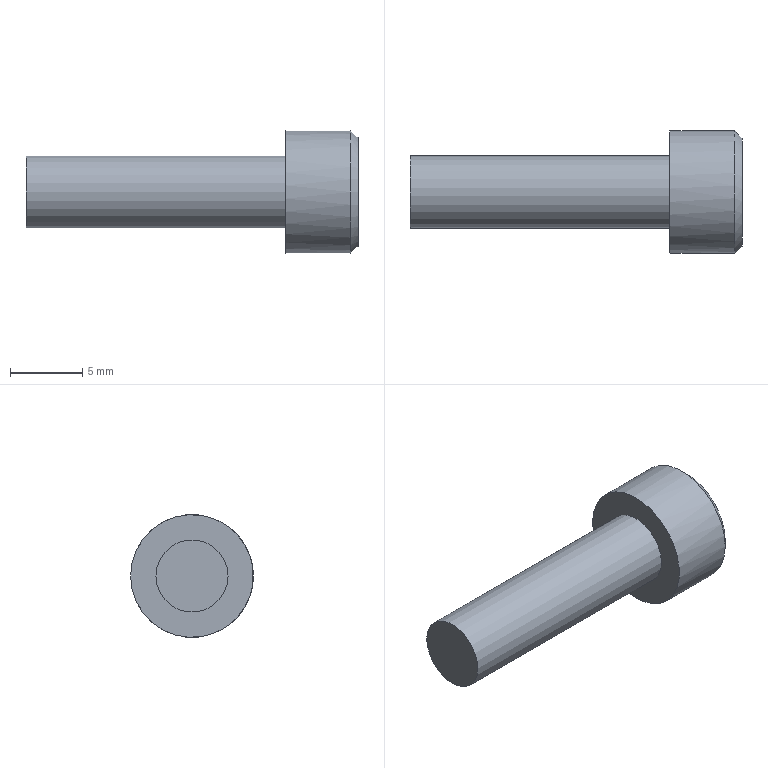Part | NX | features 5003_312_CB5-18 2 | 1 solid | 19 faces | box 23 x 8.5 x 8.5 mm | volume 594.272 mm3 | plane 15 | cylinder 2 | cone 2 | commonest cylinder face diameters 5 x1 8.5 x1
STEP:
#1=CARTESIAN_POINT('',(227.825,81.75,-47.));
#2=VERTEX_POINT('',#1);
#3=CARTESIAN_POINT('',(227.825,85.5,-47.));
#4=DIRECTION('',(-1.,0.,0.));
#5=DIRECTION('',(0.,-1.,0.));
#6=AXIS2_PLACEMENT_3D('',#3,#4,#5);
#7=CIRCLE('',#6,3.75);
#8=EDGE_CURVE('',#2,#2,#7,.F.);
#9=ORIENTED_EDGE('',*,*,#8,.T.);
#10=EDGE_LOOP('',(#9));
#11=FACE_BOUND('',#10,.T.);
#12=CARTESIAN_POINT('',(227.825,85.5,-49.309));
#13=VERTEX_POINT('',#12);
#14=CARTESIAN_POINT('',(227.825,87.5,-48.155));
#15=VERTEX_POINT('',#14);
#16=CARTESIAN_POINT('',(227.825,85.5,-49.309));
#17=DIRECTION('',(0.,0.866,0.5));
#18=VECTOR('',#17,1000.);
#19=LINE('',#16,#18);
#20=EDGE_CURVE('',#13,#15,#19,.T.);
#21=ORIENTED_EDGE('',*,*,#20,.F.);
#22=CARTESIAN_POINT('',(227.825,83.5,-48.155));
#23=VERTEX_POINT('',#22);
#24=CARTESIAN_POINT('',(227.825,83.5,-48.155));
#25=DIRECTION('',(0.,0.866,-0.5));
#26=VECTOR('',#25,1000.);
#27=LINE('',#24,#26);
#28=EDGE_CURVE('',#23,#13,#27,.T.);
#29=ORIENTED_EDGE('',*,*,#28,.F.);
#30=CARTESIAN_POINT('',(227.825,83.5,-45.845));
#31=VERTEX_POINT('',#30);
#32=CARTESIAN_POINT('',(227.825,83.5,-45.845));
#33=DIRECTION('',(0.,0.,-1.));
#34=VECTOR('',#33,1000.);
#35=LINE('',#32,#34);
#36=EDGE_CURVE('',#31,#23,#35,.T.);
#37=ORIENTED_EDGE('',*,*,#36,.F.);
#38=CARTESIAN_POINT('',(227.825,85.5,-44.691));
#39=VERTEX_POINT('',#38);
#40=CARTESIAN_POINT('',(227.825,85.5,-44.691));
#41=DIRECTION('',(0.,-0.866,-0.5));
#42=VECTOR('',#41,1000.);
#43=LINE('',#40,#42);
#44=EDGE_CURVE('',#39,#31,#43,.T.);
#45=ORIENTED_EDGE('',*,*,#44,.F.);
#46=CARTESIAN_POINT('',(227.825,87.5,-45.845));
#47=VERTEX_POINT('',#46);
#48=CARTESIAN_POINT('',(227.825,87.5,-45.845));
#49=DIRECTION('',(0.,-0.866,0.5));
#50=VECTOR('',#49,1000.);
#51=LINE('',#48,#50);
#52=EDGE_CURVE('',#47,#39,#51,.T.);
#53=ORIENTED_EDGE('',*,*,#52,.F.);
#54=CARTESIAN_POINT('',(227.825,87.5,-48.155));
#55=DIRECTION('',(0.,0.,1.));
#56=VECTOR('',#55,1000.);
#57=LINE('',#54,#56);
#58=EDGE_CURVE('',#15,#47,#57,.T.);
#59=ORIENTED_EDGE('',*,*,#58,.F.);
#60=EDGE_LOOP('',(#21,#29,#37,#45,#53,#59));
#61=FACE_BOUND('',#60,.T.);
#62=CARTESIAN_POINT('',(227.825,85.5,-42.75));
#63=DIRECTION('',(-1.,0.,0.));
#64=DIRECTION('',(0.,-1.,0.));
#65=AXIS2_PLACEMENT_3D('',#62,#63,#64);
#66=PLANE('',#65);
#67=ADVANCED_FACE('',(#11,#61),#66,.F.);
#68=CARTESIAN_POINT('',(204.825,88.,-47.));
#69=VERTEX_POINT('',#68);
#70=CARTESIAN_POINT('',(204.825,85.5,-47.));
#71=DIRECTION('',(1.,0.,0.));
#72=DIRECTION('',(0.,1.,0.));
#73=AXIS2_PLACEMENT_3D('',#70,#71,#72);
#74=CIRCLE('',#73,2.5);
#75=EDGE_CURVE('',#69,#69,#74,.T.);
#76=ORIENTED_EDGE('',*,*,#75,.F.);
#77=EDGE_LOOP('',(#76));
#78=FACE_BOUND('',#77,.T.);
#79=CARTESIAN_POINT('',(204.825,85.5,-47.));
#80=DIRECTION('',(1.,0.,0.));
#81=DIRECTION('',(0.,1.,0.));
#82=AXIS2_PLACEMENT_3D('',#79,#80,#81);
#83=PLANE('',#82);
#84=ADVANCED_FACE('',(#78),#83,.F.);
#85=CARTESIAN_POINT('',(222.825,88.,-47.));
#86=VERTEX_POINT('',#85);
#87=CARTESIAN_POINT('',(222.825,85.5,-47.));
#88=DIRECTION('',(1.,0.,0.));
#89=DIRECTION('',(0.,1.,0.));
#90=AXIS2_PLACEMENT_3D('',#87,#88,#89);
#91=CIRCLE('',#90,2.5);
#92=EDGE_CURVE('',#86,#86,#91,.T.);
#93=ORIENTED_EDGE('',*,*,#92,.F.);
#94=EDGE_LOOP('',(#93));
#95=FACE_BOUND('',#94,.T.);
#96=ORIENTED_EDGE('',*,*,#75,.T.);
#97=EDGE_LOOP('',(#96));
#98=FACE_BOUND('',#97,.T.);
#99=CARTESIAN_POINT('',(227.825,85.5,-47.));
#100=DIRECTION('',(1.,0.,0.));
#101=DIRECTION('',(0.,1.,0.));
#102=AXIS2_PLACEMENT_3D('',#99,#100,#101);
#103=CYLINDRICAL_SURFACE('',#102,2.5);
#104=ADVANCED_FACE('',(#95,#98),#103,.T.);
#105=CARTESIAN_POINT('',(222.825,89.75,-47.));
#106=VERTEX_POINT('',#105);
#107=CARTESIAN_POINT('',(222.825,85.5,-47.));
#108=DIRECTION('',(1.,0.,0.));
#109=DIRECTION('',(0.,1.,0.));
#110=AXIS2_PLACEMENT_3D('',#107,#108,#109);
#111=CIRCLE('',#110,4.25);
#112=EDGE_CURVE('',#106,#106,#111,.T.);
#113=ORIENTED_EDGE('',*,*,#112,.F.);
#114=EDGE_LOOP('',(#113));
#115=FACE_BOUND('',#114,.T.);
#116=ORIENTED_EDGE('',*,*,#92,.T.);
#117=EDGE_LOOP('',(#116));
#118=FACE_BOUND('',#117,.T.);
#119=CARTESIAN_POINT('',(222.825,85.5,-44.5));
#120=DIRECTION('',(1.,0.,0.));
#121=DIRECTION('',(0.,1.,0.));
#122=AXIS2_PLACEMENT_3D('',#119,#120,#121);
#123=PLANE('',#122);
#124=ADVANCED_FACE('',(#115,#118),#123,.F.);
#125=CARTESIAN_POINT('',(227.325,81.25,-47.));
#126=VERTEX_POINT('',#125);
#127=CARTESIAN_POINT('',(227.325,85.5,-47.));
#128=DIRECTION('',(-1.,0.,0.));
#129=DIRECTION('',(0.,-1.,0.));
#130=AXIS2_PLACEMENT_3D('',#127,#128,#129);
#131=CIRCLE('',#130,4.25);
#132=EDGE_CURVE('',#126,#126,#131,.T.);
#133=ORIENTED_EDGE('',*,*,#132,.T.);
#134=EDGE_LOOP('',(#133));
#135=FACE_BOUND('',#134,.T.);
#136=ORIENTED_EDGE('',*,*,#112,.T.);
#137=EDGE_LOOP('',(#136));
#138=FACE_BOUND('',#137,.T.);
#139=CARTESIAN_POINT('',(227.825,85.5,-47.));
#140=DIRECTION('',(1.,0.,0.));
#141=DIRECTION('',(0.,1.,0.));
#142=AXIS2_PLACEMENT_3D('',#139,#140,#141);
#143=CYLINDRICAL_SURFACE('',#142,4.25);
#144=ADVANCED_FACE('',(#135,#138),#143,.T.);
#145=ORIENTED_EDGE('',*,*,#132,.F.);
#146=EDGE_LOOP('',(#145));
#147=FACE_BOUND('',#146,.T.);
#148=ORIENTED_EDGE('',*,*,#8,.F.);
#149=EDGE_LOOP('',(#148));
#150=FACE_BOUND('',#149,.T.);
#151=CARTESIAN_POINT('',(227.825,85.5,-47.));
#152=DIRECTION('',(-1.,0.,0.));
#153=DIRECTION('',(0.,-1.,0.));
#154=AXIS2_PLACEMENT_3D('',#151,#152,#153);
#155=CONICAL_SURFACE('',#154,3.75,0.7854);
#156=ADVANCED_FACE('',(#147,#150),#155,.T.);
#157=CARTESIAN_POINT('',(225.325,83.5,-48.155));
#158=VERTEX_POINT('',#157);
#159=CARTESIAN_POINT('',(225.325,84.5,-48.732));
#160=VERTEX_POINT('',#159);
#161=CARTESIAN_POINT('',(225.325,83.5,-48.155));
#162=DIRECTION('',(0.,0.866,-0.5));
#163=VECTOR('',#162,1000.);
#164=LINE('',#161,#163);
#165=EDGE_CURVE('',#158,#160,#164,.T.);
#166=ORIENTED_EDGE('',*,*,#165,.F.);
#167=CARTESIAN_POINT('',(225.325,83.5,-48.155));
#168=DIRECTION('',(1.,0.,0.));
#169=VECTOR('',#168,1000.);
#170=LINE('',#167,#169);
#171=EDGE_CURVE('',#158,#23,#170,.T.);
#172=ORIENTED_EDGE('',*,*,#171,.T.);
#173=ORIENTED_EDGE('',*,*,#28,.T.);
#174=CARTESIAN_POINT('',(225.325,85.5,-49.309));
#175=VERTEX_POINT('',#174);
#176=CARTESIAN_POINT('',(225.325,85.5,-49.309));
#177=DIRECTION('',(1.,0.,0.));
#178=VECTOR('',#177,1000.);
#179=LINE('',#176,#178);
#180=EDGE_CURVE('',#175,#13,#179,.T.);
#181=ORIENTED_EDGE('',*,*,#180,.F.);
#182=CARTESIAN_POINT('',(225.325,83.5,-48.155));
#183=DIRECTION('',(0.,0.866,-0.5));
#184=VECTOR('',#183,1000.);
#185=LINE('',#182,#184);
#186=EDGE_CURVE('',#160,#175,#185,.T.);
#187=ORIENTED_EDGE('',*,*,#186,.F.);
#188=EDGE_LOOP('',(#166,#172,#173,#181,#187));
#189=FACE_BOUND('',#188,.T.);
#190=CARTESIAN_POINT('',(225.325,83.5,-48.155));
#191=DIRECTION('',(0.,-0.5,-0.866));
#192=DIRECTION('',(0.,-0.866,0.5));
#193=AXIS2_PLACEMENT_3D('',#190,#191,#192);
#194=PLANE('',#193);
#195=ADVANCED_FACE('',(#189),#194,.F.);
#196=CARTESIAN_POINT('',(225.325,83.5,-45.845));
#197=VERTEX_POINT('',#196);
#198=CARTESIAN_POINT('',(225.325,83.5,-47.));
#199=VERTEX_POINT('',#198);
#200=CARTESIAN_POINT('',(225.325,83.5,-45.845));
#201=DIRECTION('',(0.,0.,-1.));
#202=VECTOR('',#201,1000.);
#203=LINE('',#200,#202);
#204=EDGE_CURVE('',#197,#199,#203,.T.);
#205=ORIENTED_EDGE('',*,*,#204,.F.);
#206=CARTESIAN_POINT('',(225.325,83.5,-45.845));
#207=DIRECTION('',(1.,0.,0.));
#208=VECTOR('',#207,1000.);
#209=LINE('',#206,#208);
#210=EDGE_CURVE('',#197,#31,#209,.T.);
#211=ORIENTED_EDGE('',*,*,#210,.T.);
#212=ORIENTED_EDGE('',*,*,#36,.T.);
#213=ORIENTED_EDGE('',*,*,#171,.F.);
#214=CARTESIAN_POINT('',(225.325,83.5,-45.845));
#215=DIRECTION('',(0.,0.,-1.));
#216=VECTOR('',#215,1000.);
#217=LINE('',#214,#216);
#218=EDGE_CURVE('',#199,#158,#217,.T.);
#219=ORIENTED_EDGE('',*,*,#218,.F.);
#220=EDGE_LOOP('',(#205,#211,#212,#213,#219));
#221=FACE_BOUND('',#220,.T.);
#222=CARTESIAN_POINT('',(225.325,83.5,-45.845));
#223=DIRECTION('',(0.,-1.,0.));
#224=DIRECTION('',(1.,0.,0.));
#225=AXIS2_PLACEMENT_3D('',#222,#223,#224);
#226=PLANE('',#225);
#227=ADVANCED_FACE('',(#221),#226,.F.);
#228=CARTESIAN_POINT('',(225.325,85.5,-44.691));
#229=VERTEX_POINT('',#228);
#230=CARTESIAN_POINT('',(225.325,84.5,-45.268));
#231=VERTEX_POINT('',#230);
#232=CARTESIAN_POINT('',(225.325,85.5,-44.691));
#233=DIRECTION('',(0.,-0.866,-0.5));
#234=VECTOR('',#233,1000.);
#235=LINE('',#232,#234);
#236=EDGE_CURVE('',#229,#231,#235,.T.);
#237=ORIENTED_EDGE('',*,*,#236,.F.);
#238=CARTESIAN_POINT('',(225.325,85.5,-44.691));
#239=DIRECTION('',(1.,0.,0.));
#240=VECTOR('',#239,1000.);
#241=LINE('',#238,#240);
#242=EDGE_CURVE('',#229,#39,#241,.T.);
#243=ORIENTED_EDGE('',*,*,#242,.T.);
#244=ORIENTED_EDGE('',*,*,#44,.T.);
#245=ORIENTED_EDGE('',*,*,#210,.F.);
#246=CARTESIAN_POINT('',(225.325,85.5,-44.691));
#247=DIRECTION('',(0.,-0.866,-0.5));
#248=VECTOR('',#247,1000.);
#249=LINE('',#246,#248);
#250=EDGE_CURVE('',#231,#197,#249,.T.);
#251=ORIENTED_EDGE('',*,*,#250,.F.);
#252=EDGE_LOOP('',(#237,#243,#244,#245,#251));
#253=FACE_BOUND('',#252,.T.);
#254=CARTESIAN_POINT('',(225.325,85.5,-44.691));
#255=DIRECTION('',(0.,-0.5,0.866));
#256=DIRECTION('',(0.,0.866,0.5));
#257=AXIS2_PLACEMENT_3D('',#254,#255,#256);
#258=PLANE('',#257);
#259=ADVANCED_FACE('',(#253),#258,.F.);
#260=CARTESIAN_POINT('',(225.325,87.5,-45.845));
#261=VERTEX_POINT('',#260);
#262=CARTESIAN_POINT('',(225.325,86.5,-45.268));
#263=VERTEX_POINT('',#262);
#264=CARTESIAN_POINT('',(225.325,87.5,-45.845));
#265=DIRECTION('',(0.,-0.866,0.5));
#266=VECTOR('',#265,1000.);
#267=LINE('',#264,#266);
#268=EDGE_CURVE('',#261,#263,#267,.T.);
#269=ORIENTED_EDGE('',*,*,#268,.F.);
#270=CARTESIAN_POINT('',(225.325,87.5,-45.845));
#271=DIRECTION('',(1.,0.,0.));
#272=VECTOR('',#271,1000.);
#273=LINE('',#270,#272);
#274=EDGE_CURVE('',#261,#47,#273,.T.);
#275=ORIENTED_EDGE('',*,*,#274,.T.);
#276=ORIENTED_EDGE('',*,*,#52,.T.);
#277=ORIENTED_EDGE('',*,*,#242,.F.);
#278=CARTESIAN_POINT('',(225.325,87.5,-45.845));
#279=DIRECTION('',(0.,-0.866,0.5));
#280=VECTOR('',#279,1000.);
#281=LINE('',#278,#280);
#282=EDGE_CURVE('',#263,#229,#281,.T.);
#283=ORIENTED_EDGE('',*,*,#282,.F.);
#284=EDGE_LOOP('',(#269,#275,#276,#277,#283));
#285=FACE_BOUND('',#284,.T.);
#286=CARTESIAN_POINT('',(225.325,87.5,-45.845));
#287=DIRECTION('',(0.,0.5,0.866));
#288=DIRECTION('',(0.,0.866,-0.5));
#289=AXIS2_PLACEMENT_3D('',#286,#287,#288);
#290=PLANE('',#289);
#291=ADVANCED_FACE('',(#285),#290,.F.);
#292=CARTESIAN_POINT('',(225.325,87.5,-48.155));
#293=VERTEX_POINT('',#292);
#294=CARTESIAN_POINT('',(225.325,87.5,-47.));
#295=VERTEX_POINT('',#294);
#296=CARTESIAN_POINT('',(225.325,87.5,-48.155));
#297=DIRECTION('',(0.,0.,1.));
#298=VECTOR('',#297,1000.);
#299=LINE('',#296,#298);
#300=EDGE_CURVE('',#293,#295,#299,.T.);
#301=ORIENTED_EDGE('',*,*,#300,.F.);
#302=CARTESIAN_POINT('',(225.325,87.5,-48.155));
#303=DIRECTION('',(1.,0.,0.));
#304=VECTOR('',#303,1000.);
#305=LINE('',#302,#304);
#306=EDGE_CURVE('',#293,#15,#305,.T.);
#307=ORIENTED_EDGE('',*,*,#306,.T.);
#308=ORIENTED_EDGE('',*,*,#58,.T.);
#309=ORIENTED_EDGE('',*,*,#274,.F.);
#310=CARTESIAN_POINT('',(225.325,87.5,-48.155));
#311=DIRECTION('',(0.,0.,1.));
#312=VECTOR('',#311,1000.);
#313=LINE('',#310,#312);
#314=EDGE_CURVE('',#295,#261,#313,.T.);
#315=ORIENTED_EDGE('',*,*,#314,.F.);
#316=EDGE_LOOP('',(#301,#307,#308,#309,#315));
#317=FACE_BOUND('',#316,.T.);
#318=CARTESIAN_POINT('',(225.325,87.5,-48.155));
#319=DIRECTION('',(0.,1.,0.));
#320=DIRECTION('',(0.,0.,-1.));
#321=AXIS2_PLACEMENT_3D('',#318,#319,#320);
#322=PLANE('',#321);
#323=ADVANCED_FACE('',(#317),#322,.F.);
#324=CARTESIAN_POINT('',(225.325,86.5,-48.732));
#325=VERTEX_POINT('',#324);
#326=CARTESIAN_POINT('',(225.325,85.5,-49.309));
#327=DIRECTION('',(0.,0.866,0.5));
#328=VECTOR('',#327,1000.);
#329=LINE('',#326,#328);
#330=EDGE_CURVE('',#175,#325,#329,.T.);
#331=ORIENTED_EDGE('',*,*,#330,.F.);
#332=ORIENTED_EDGE('',*,*,#180,.T.);
#333=ORIENTED_EDGE('',*,*,#20,.T.);
#334=ORIENTED_EDGE('',*,*,#306,.F.);
#335=CARTESIAN_POINT('',(225.325,85.5,-49.309));
#336=DIRECTION('',(0.,0.866,0.5));
#337=VECTOR('',#336,1000.);
#338=LINE('',#335,#337);
#339=EDGE_CURVE('',#325,#293,#338,.T.);
#340=ORIENTED_EDGE('',*,*,#339,.F.);
#341=EDGE_LOOP('',(#331,#332,#333,#334,#340));
#342=FACE_BOUND('',#341,.T.);
#343=CARTESIAN_POINT('',(225.325,85.5,-49.309));
#344=DIRECTION('',(0.,0.5,-0.866));
#345=DIRECTION('',(0.,-0.866,-0.5));
#346=AXIS2_PLACEMENT_3D('',#343,#344,#345);
#347=PLANE('',#346);
#348=ADVANCED_FACE('',(#342),#347,.F.);
#349=ORIENTED_EDGE('',*,*,#314,.T.);
#350=ORIENTED_EDGE('',*,*,#268,.T.);
#351=CARTESIAN_POINT('',(225.325,85.5,-47.));
#352=DIRECTION('',(1.,0.,0.));
#353=DIRECTION('',(0.,0.,-1.));
#354=AXIS2_PLACEMENT_3D('',#351,#352,#353);
#355=CIRCLE('',#354,2.);
#356=EDGE_CURVE('',#295,#263,#355,.T.);
#357=ORIENTED_EDGE('',*,*,#356,.F.);
#358=EDGE_LOOP('',(#349,#350,#357));
#359=FACE_BOUND('',#358,.T.);
#360=CARTESIAN_POINT('',(225.325,85.5,-47.));
#361=DIRECTION('',(1.,0.,0.));
#362=DIRECTION('',(0.,1.,0.));
#363=AXIS2_PLACEMENT_3D('',#360,#361,#362);
#364=PLANE('',#363);
#365=ADVANCED_FACE('',(#359),#364,.T.);
#366=ORIENTED_EDGE('',*,*,#282,.T.);
#367=ORIENTED_EDGE('',*,*,#236,.T.);
#368=CARTESIAN_POINT('',(225.325,85.5,-47.));
#369=DIRECTION('',(1.,0.,0.));
#370=DIRECTION('',(0.,0.,-1.));
#371=AXIS2_PLACEMENT_3D('',#368,#369,#370);
#372=CIRCLE('',#371,2.);
#373=EDGE_CURVE('',#263,#231,#372,.T.);
#374=ORIENTED_EDGE('',*,*,#373,.F.);
#375=EDGE_LOOP('',(#366,#367,#374));
#376=FACE_BOUND('',#375,.T.);
#377=CARTESIAN_POINT('',(225.325,85.5,-47.));
#378=DIRECTION('',(1.,0.,0.));
#379=DIRECTION('',(0.,1.,0.));
#380=AXIS2_PLACEMENT_3D('',#377,#378,#379);
#381=PLANE('',#380);
#382=ADVANCED_FACE('',(#376),#381,.T.);
#383=ORIENTED_EDGE('',*,*,#250,.T.);
#384=ORIENTED_EDGE('',*,*,#204,.T.);
#385=CARTESIAN_POINT('',(225.325,85.5,-47.));
#386=DIRECTION('',(1.,0.,0.));
#387=DIRECTION('',(0.,0.,-1.));
#388=AXIS2_PLACEMENT_3D('',#385,#386,#387);
#389=CIRCLE('',#388,2.);
#390=EDGE_CURVE('',#231,#199,#389,.T.);
#391=ORIENTED_EDGE('',*,*,#390,.F.);
#392=EDGE_LOOP('',(#383,#384,#391));
#393=FACE_BOUND('',#392,.T.);
#394=CARTESIAN_POINT('',(225.325,85.5,-47.));
#395=DIRECTION('',(1.,0.,0.));
#396=DIRECTION('',(0.,1.,0.));
#397=AXIS2_PLACEMENT_3D('',#394,#395,#396);
#398=PLANE('',#397);
#399=ADVANCED_FACE('',(#393),#398,.T.);
#400=ORIENTED_EDGE('',*,*,#218,.T.);
#401=ORIENTED_EDGE('',*,*,#165,.T.);
#402=CARTESIAN_POINT('',(225.325,85.5,-47.));
#403=DIRECTION('',(1.,0.,0.));
#404=DIRECTION('',(0.,0.,-1.));
#405=AXIS2_PLACEMENT_3D('',#402,#403,#404);
#406=CIRCLE('',#405,2.);
#407=EDGE_CURVE('',#199,#160,#406,.T.);
#408=ORIENTED_EDGE('',*,*,#407,.F.);
#409=EDGE_LOOP('',(#400,#401,#408));
#410=FACE_BOUND('',#409,.T.);
#411=CARTESIAN_POINT('',(225.325,85.5,-47.));
#412=DIRECTION('',(1.,0.,0.));
#413=DIRECTION('',(0.,1.,0.));
#414=AXIS2_PLACEMENT_3D('',#411,#412,#413);
#415=PLANE('',#414);
#416=ADVANCED_FACE('',(#410),#415,.T.);
#417=ORIENTED_EDGE('',*,*,#186,.T.);
#418=ORIENTED_EDGE('',*,*,#330,.T.);
#419=CARTESIAN_POINT('',(225.325,85.5,-47.));
#420=DIRECTION('',(1.,0.,0.));
#421=DIRECTION('',(0.,0.,-1.));
#422=AXIS2_PLACEMENT_3D('',#419,#420,#421);
#423=CIRCLE('',#422,2.);
#424=EDGE_CURVE('',#160,#325,#423,.T.);
#425=ORIENTED_EDGE('',*,*,#424,.F.);
#426=EDGE_LOOP('',(#417,#418,#425));
#427=FACE_BOUND('',#426,.T.);
#428=CARTESIAN_POINT('',(225.325,85.5,-47.));
#429=DIRECTION('',(1.,0.,0.));
#430=DIRECTION('',(0.,1.,0.));
#431=AXIS2_PLACEMENT_3D('',#428,#429,#430);
#432=PLANE('',#431);
#433=ADVANCED_FACE('',(#427),#432,.T.);
#434=ORIENTED_EDGE('',*,*,#339,.T.);
#435=ORIENTED_EDGE('',*,*,#300,.T.);
#436=CARTESIAN_POINT('',(225.325,85.5,-47.));
#437=DIRECTION('',(1.,0.,0.));
#438=DIRECTION('',(0.,0.,-1.));
#439=AXIS2_PLACEMENT_3D('',#436,#437,#438);
#440=CIRCLE('',#439,2.);
#441=EDGE_CURVE('',#325,#295,#440,.T.);
#442=ORIENTED_EDGE('',*,*,#441,.F.);
#443=EDGE_LOOP('',(#434,#435,#442));
#444=FACE_BOUND('',#443,.T.);
#445=CARTESIAN_POINT('',(225.325,85.5,-47.));
#446=DIRECTION('',(1.,0.,0.));
#447=DIRECTION('',(0.,1.,0.));
#448=AXIS2_PLACEMENT_3D('',#445,#446,#447);
#449=PLANE('',#448);
#450=ADVANCED_FACE('',(#444),#449,.T.);
#451=ORIENTED_EDGE('',*,*,#441,.T.);
#452=ORIENTED_EDGE('',*,*,#356,.T.);
#453=ORIENTED_EDGE('',*,*,#373,.T.);
#454=ORIENTED_EDGE('',*,*,#390,.T.);
#455=ORIENTED_EDGE('',*,*,#407,.T.);
#456=ORIENTED_EDGE('',*,*,#424,.T.);
#457=EDGE_LOOP('',(#451,#452,#453,#454,#455,#456));
#458=FACE_BOUND('',#457,.T.);
#459=CARTESIAN_POINT('',(224.123,85.5,-47.));
#460=VERTEX_POINT('',#459);
#461=VERTEX_LOOP('',#460);
#462=FACE_BOUND('',#461,.T.);
#463=CARTESIAN_POINT('',(224.123,85.5,-47.));
#464=DIRECTION('',(1.,0.,0.));
#465=DIRECTION('',(0.,0.,-1.));
#466=AXIS2_PLACEMENT_3D('',#463,#464,#465);
#467=CONICAL_SURFACE('',#466,0.,1.03);
#468=ADVANCED_FACE('',(#458,#462),#467,.F.);
#469=CLOSED_SHELL('',(#67,#84,#104,#124,#144,#156,#195,#227,#259,#291,#323,#348,#365,#382,#399,#416,#433,#450,#468));
#470=MANIFOLD_SOLID_BREP('',#469);
#471=(LENGTH_UNIT()NAMED_UNIT(*)SI_UNIT(.MILLI.,.METRE.));
#472=UNCERTAINTY_MEASURE_WITH_UNIT(LENGTH_MEASURE(0.00001),#471,'','');
#473=(NAMED_UNIT(*)PLANE_ANGLE_UNIT()SI_UNIT($,.RADIAN.));
#474=(NAMED_UNIT(*)SI_UNIT($,.STERADIAN.)SOLID_ANGLE_UNIT());
#475=(GEOMETRIC_REPRESENTATION_CONTEXT(3)GLOBAL_UNCERTAINTY_ASSIGNED_CONTEXT((#472))GLOBAL_UNIT_ASSIGNED_CONTEXT((#471,#473,#474))REPRESENTATION_CONTEXT('',''));
#476=ADVANCED_BREP_SHAPE_REPRESENTATION('',(#470),#475);